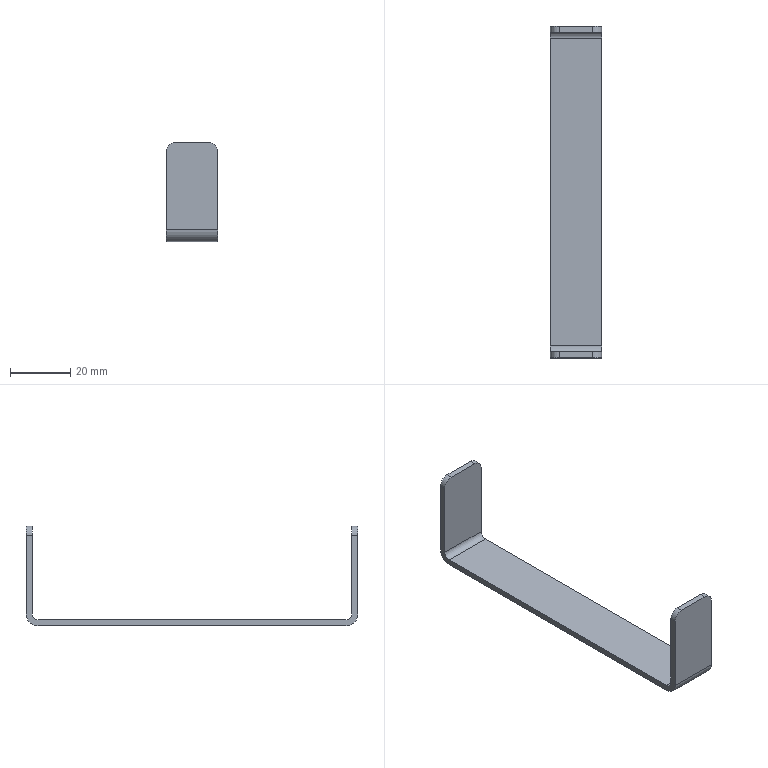Part | NX | features solid 2 | 1 solid | 18 faces | box 17 x 110 x 33 mm | volume 5745 mm3 | plane 10 | cylinder 8 | commonest cylinder face diameters 6 x4 4 x2 8 x2
STEP:
#1=CARTESIAN_POINT('',(1091.5,-530.,943.5));
#2=VERTEX_POINT('',#1);
#3=CARTESIAN_POINT('',(1094.5,-530.,946.5));
#4=VERTEX_POINT('',#3);
#5=CARTESIAN_POINT('',(1094.5,-530.,943.5));
#6=DIRECTION('',(0.,1.,0.));
#7=DIRECTION('',(0.,0.,1.));
#8=AXIS2_PLACEMENT_3D('',#5,#6,#7);
#9=CIRCLE('',#8,3.);
#10=EDGE_CURVE('',#2,#4,#9,.T.);
#11=ORIENTED_EDGE('',*,*,#10,.F.);
#12=CARTESIAN_POINT('',(1091.5,-532.,943.5));
#13=VERTEX_POINT('',#12);
#14=CARTESIAN_POINT('',(1091.5,-422.,943.5));
#15=DIRECTION('',(0.,1.,0.));
#16=VECTOR('',#15,1000.);
#17=LINE('',#14,#16);
#18=EDGE_CURVE('',#13,#2,#17,.T.);
#19=ORIENTED_EDGE('',*,*,#18,.F.);
#20=CARTESIAN_POINT('',(1094.5,-532.,946.5));
#21=VERTEX_POINT('',#20);
#22=CARTESIAN_POINT('',(1094.5,-532.,943.5));
#23=DIRECTION('',(0.,-1.,0.));
#24=DIRECTION('',(0.,0.,1.));
#25=AXIS2_PLACEMENT_3D('',#22,#23,#24);
#26=CIRCLE('',#25,3.);
#27=EDGE_CURVE('',#21,#13,#26,.T.);
#28=ORIENTED_EDGE('',*,*,#27,.F.);
#29=CARTESIAN_POINT('',(1094.5,-532.,946.5));
#30=DIRECTION('',(0.,-1.,0.));
#31=VECTOR('',#30,1000.);
#32=LINE('',#29,#31);
#33=EDGE_CURVE('',#4,#21,#32,.T.);
#34=ORIENTED_EDGE('',*,*,#33,.F.);
#35=EDGE_LOOP('',(#11,#19,#28,#34));
#36=FACE_BOUND('',#35,.T.);
#37=CARTESIAN_POINT('',(1094.5,-532.,943.5));
#38=DIRECTION('',(0.,1.,0.));
#39=DIRECTION('',(0.,0.,-1.));
#40=AXIS2_PLACEMENT_3D('',#37,#38,#39);
#41=CYLINDRICAL_SURFACE('',#40,3.);
#42=ADVANCED_FACE('',(#36),#41,.T.);
#43=CARTESIAN_POINT('',(1105.5,-530.,946.5));
#44=VERTEX_POINT('',#43);
#45=CARTESIAN_POINT('',(1108.5,-530.,943.5));
#46=VERTEX_POINT('',#45);
#47=CARTESIAN_POINT('',(1105.5,-530.,943.5));
#48=DIRECTION('',(0.,1.,0.));
#49=DIRECTION('',(0.,0.,1.));
#50=AXIS2_PLACEMENT_3D('',#47,#48,#49);
#51=CIRCLE('',#50,3.);
#52=EDGE_CURVE('',#44,#46,#51,.T.);
#53=ORIENTED_EDGE('',*,*,#52,.F.);
#54=CARTESIAN_POINT('',(1105.5,-532.,946.5));
#55=VERTEX_POINT('',#54);
#56=CARTESIAN_POINT('',(1105.5,-532.,946.5));
#57=DIRECTION('',(0.,1.,0.));
#58=VECTOR('',#57,1000.);
#59=LINE('',#56,#58);
#60=EDGE_CURVE('',#55,#44,#59,.T.);
#61=ORIENTED_EDGE('',*,*,#60,.F.);
#62=CARTESIAN_POINT('',(1108.5,-532.,943.5));
#63=VERTEX_POINT('',#62);
#64=CARTESIAN_POINT('',(1105.5,-532.,943.5));
#65=DIRECTION('',(0.,-1.,0.));
#66=DIRECTION('',(0.,0.,1.));
#67=AXIS2_PLACEMENT_3D('',#64,#65,#66);
#68=CIRCLE('',#67,3.);
#69=EDGE_CURVE('',#63,#55,#68,.T.);
#70=ORIENTED_EDGE('',*,*,#69,.F.);
#71=CARTESIAN_POINT('',(1108.5,-532.,943.5));
#72=DIRECTION('',(0.,-1.,0.));
#73=VECTOR('',#72,1000.);
#74=LINE('',#71,#73);
#75=EDGE_CURVE('',#46,#63,#74,.T.);
#76=ORIENTED_EDGE('',*,*,#75,.F.);
#77=EDGE_LOOP('',(#53,#61,#70,#76));
#78=FACE_BOUND('',#77,.T.);
#79=CARTESIAN_POINT('',(1105.5,-532.,943.5));
#80=DIRECTION('',(0.,-1.,0.));
#81=DIRECTION('',(0.,0.,1.));
#82=AXIS2_PLACEMENT_3D('',#79,#80,#81);
#83=CYLINDRICAL_SURFACE('',#82,3.);
#84=ADVANCED_FACE('',(#78),#83,.T.);
#85=CARTESIAN_POINT('',(1094.5,-424.,946.5));
#86=VERTEX_POINT('',#85);
#87=CARTESIAN_POINT('',(1091.5,-424.,943.5));
#88=VERTEX_POINT('',#87);
#89=CARTESIAN_POINT('',(1094.5,-424.,943.5));
#90=DIRECTION('',(0.,-1.,0.));
#91=DIRECTION('',(0.,0.,-1.));
#92=AXIS2_PLACEMENT_3D('',#89,#90,#91);
#93=CIRCLE('',#92,3.);
#94=EDGE_CURVE('',#86,#88,#93,.T.);
#95=ORIENTED_EDGE('',*,*,#94,.F.);
#96=CARTESIAN_POINT('',(1094.5,-422.,946.5));
#97=VERTEX_POINT('',#96);
#98=CARTESIAN_POINT('',(1094.5,-422.,946.5));
#99=DIRECTION('',(0.,-1.,0.));
#100=VECTOR('',#99,1000.);
#101=LINE('',#98,#100);
#102=EDGE_CURVE('',#97,#86,#101,.T.);
#103=ORIENTED_EDGE('',*,*,#102,.F.);
#104=CARTESIAN_POINT('',(1091.5,-422.,943.5));
#105=VERTEX_POINT('',#104);
#106=CARTESIAN_POINT('',(1094.5,-422.,943.5));
#107=DIRECTION('',(0.,1.,0.));
#108=DIRECTION('',(0.,0.,-1.));
#109=AXIS2_PLACEMENT_3D('',#106,#107,#108);
#110=CIRCLE('',#109,3.);
#111=EDGE_CURVE('',#105,#97,#110,.T.);
#112=ORIENTED_EDGE('',*,*,#111,.F.);
#113=CARTESIAN_POINT('',(1091.5,-422.,943.5));
#114=DIRECTION('',(0.,1.,0.));
#115=VECTOR('',#114,1000.);
#116=LINE('',#113,#115);
#117=EDGE_CURVE('',#88,#105,#116,.T.);
#118=ORIENTED_EDGE('',*,*,#117,.F.);
#119=EDGE_LOOP('',(#95,#103,#112,#118));
#120=FACE_BOUND('',#119,.T.);
#121=CARTESIAN_POINT('',(1094.5,-422.,943.5));
#122=DIRECTION('',(0.,1.,0.));
#123=DIRECTION('',(0.,0.,-1.));
#124=AXIS2_PLACEMENT_3D('',#121,#122,#123);
#125=CYLINDRICAL_SURFACE('',#124,3.);
#126=ADVANCED_FACE('',(#120),#125,.T.);
#127=CARTESIAN_POINT('',(1108.5,-424.,943.5));
#128=VERTEX_POINT('',#127);
#129=CARTESIAN_POINT('',(1105.5,-424.,946.5));
#130=VERTEX_POINT('',#129);
#131=CARTESIAN_POINT('',(1105.5,-424.,943.5));
#132=DIRECTION('',(0.,-1.,0.));
#133=DIRECTION('',(0.,0.,-1.));
#134=AXIS2_PLACEMENT_3D('',#131,#132,#133);
#135=CIRCLE('',#134,3.);
#136=EDGE_CURVE('',#128,#130,#135,.T.);
#137=ORIENTED_EDGE('',*,*,#136,.F.);
#138=CARTESIAN_POINT('',(1108.5,-422.,943.5));
#139=VERTEX_POINT('',#138);
#140=CARTESIAN_POINT('',(1108.5,-532.,943.5));
#141=DIRECTION('',(0.,-1.,0.));
#142=VECTOR('',#141,1000.);
#143=LINE('',#140,#142);
#144=EDGE_CURVE('',#139,#128,#143,.T.);
#145=ORIENTED_EDGE('',*,*,#144,.F.);
#146=CARTESIAN_POINT('',(1105.5,-422.,946.5));
#147=VERTEX_POINT('',#146);
#148=CARTESIAN_POINT('',(1105.5,-422.,943.5));
#149=DIRECTION('',(0.,1.,0.));
#150=DIRECTION('',(0.,0.,-1.));
#151=AXIS2_PLACEMENT_3D('',#148,#149,#150);
#152=CIRCLE('',#151,3.);
#153=EDGE_CURVE('',#147,#139,#152,.T.);
#154=ORIENTED_EDGE('',*,*,#153,.F.);
#155=CARTESIAN_POINT('',(1105.5,-422.,946.5));
#156=DIRECTION('',(0.,1.,0.));
#157=VECTOR('',#156,1000.);
#158=LINE('',#155,#157);
#159=EDGE_CURVE('',#130,#147,#158,.T.);
#160=ORIENTED_EDGE('',*,*,#159,.F.);
#161=EDGE_LOOP('',(#137,#145,#154,#160));
#162=FACE_BOUND('',#161,.T.);
#163=CARTESIAN_POINT('',(1105.5,-422.,943.5));
#164=DIRECTION('',(0.,-1.,0.));
#165=DIRECTION('',(0.,0.,1.));
#166=AXIS2_PLACEMENT_3D('',#163,#164,#165);
#167=CYLINDRICAL_SURFACE('',#166,3.);
#168=ADVANCED_FACE('',(#162),#167,.T.);
#169=CARTESIAN_POINT('',(1108.5,-424.,917.5));
#170=VERTEX_POINT('',#169);
#171=CARTESIAN_POINT('',(1108.5,-424.,913.5));
#172=DIRECTION('',(0.,0.,1.));
#173=VECTOR('',#172,1000.);
#174=LINE('',#171,#173);
#175=EDGE_CURVE('',#170,#128,#174,.T.);
#176=ORIENTED_EDGE('',*,*,#175,.T.);
#177=ORIENTED_EDGE('',*,*,#136,.T.);
#178=CARTESIAN_POINT('',(1091.5,-424.,946.5));
#179=DIRECTION('',(1.,0.,0.));
#180=VECTOR('',#179,1000.);
#181=LINE('',#178,#180);
#182=EDGE_CURVE('',#86,#130,#181,.T.);
#183=ORIENTED_EDGE('',*,*,#182,.F.);
#184=ORIENTED_EDGE('',*,*,#94,.T.);
#185=CARTESIAN_POINT('',(1091.5,-424.,917.5));
#186=VERTEX_POINT('',#185);
#187=CARTESIAN_POINT('',(1091.5,-424.,913.5));
#188=DIRECTION('',(0.,0.,1.));
#189=VECTOR('',#188,1000.);
#190=LINE('',#187,#189);
#191=EDGE_CURVE('',#186,#88,#190,.T.);
#192=ORIENTED_EDGE('',*,*,#191,.F.);
#193=CARTESIAN_POINT('',(1091.5,-424.,917.5));
#194=DIRECTION('',(1.,0.,0.));
#195=VECTOR('',#194,1000.);
#196=LINE('',#193,#195);
#197=EDGE_CURVE('',#186,#170,#196,.T.);
#198=ORIENTED_EDGE('',*,*,#197,.T.);
#199=EDGE_LOOP('',(#176,#177,#183,#184,#192,#198));
#200=FACE_BOUND('',#199,.T.);
#201=CARTESIAN_POINT('',(1091.5,-424.,913.5));
#202=DIRECTION('',(0.,1.,0.));
#203=DIRECTION('',(0.,0.,-1.));
#204=AXIS2_PLACEMENT_3D('',#201,#202,#203);
#205=PLANE('',#204);
#206=ADVANCED_FACE('',(#200),#205,.F.);
#207=CARTESIAN_POINT('',(1108.5,-426.,915.5));
#208=VERTEX_POINT('',#207);
#209=CARTESIAN_POINT('',(1108.5,-426.,917.5));
#210=DIRECTION('',(1.,0.,0.));
#211=DIRECTION('',(0.,0.,-1.));
#212=AXIS2_PLACEMENT_3D('',#209,#210,#211);
#213=CIRCLE('',#212,2.);
#214=EDGE_CURVE('',#208,#170,#213,.T.);
#215=ORIENTED_EDGE('',*,*,#214,.T.);
#216=ORIENTED_EDGE('',*,*,#197,.F.);
#217=CARTESIAN_POINT('',(1091.5,-426.,915.5));
#218=VERTEX_POINT('',#217);
#219=CARTESIAN_POINT('',(1091.5,-426.,917.5));
#220=DIRECTION('',(1.,0.,0.));
#221=DIRECTION('',(0.,0.,-1.));
#222=AXIS2_PLACEMENT_3D('',#219,#220,#221);
#223=CIRCLE('',#222,2.);
#224=EDGE_CURVE('',#218,#186,#223,.T.);
#225=ORIENTED_EDGE('',*,*,#224,.F.);
#226=CARTESIAN_POINT('',(1091.5,-426.,915.5));
#227=DIRECTION('',(1.,0.,0.));
#228=VECTOR('',#227,1000.);
#229=LINE('',#226,#228);
#230=EDGE_CURVE('',#218,#208,#229,.T.);
#231=ORIENTED_EDGE('',*,*,#230,.T.);
#232=EDGE_LOOP('',(#215,#216,#225,#231));
#233=FACE_BOUND('',#232,.T.);
#234=CARTESIAN_POINT('',(1091.5,-426.,917.5));
#235=DIRECTION('',(1.,0.,0.));
#236=DIRECTION('',(0.,0.,-1.));
#237=AXIS2_PLACEMENT_3D('',#234,#235,#236);
#238=CYLINDRICAL_SURFACE('',#237,2.);
#239=ADVANCED_FACE('',(#233),#238,.F.);
#240=CARTESIAN_POINT('',(1108.5,-528.,915.5));
#241=VERTEX_POINT('',#240);
#242=CARTESIAN_POINT('',(1108.5,-532.,915.5));
#243=DIRECTION('',(0.,1.,0.));
#244=VECTOR('',#243,1000.);
#245=LINE('',#242,#244);
#246=EDGE_CURVE('',#241,#208,#245,.T.);
#247=ORIENTED_EDGE('',*,*,#246,.T.);
#248=ORIENTED_EDGE('',*,*,#230,.F.);
#249=CARTESIAN_POINT('',(1091.5,-528.,915.5));
#250=VERTEX_POINT('',#249);
#251=CARTESIAN_POINT('',(1091.5,-532.,915.5));
#252=DIRECTION('',(0.,1.,0.));
#253=VECTOR('',#252,1000.);
#254=LINE('',#251,#253);
#255=EDGE_CURVE('',#250,#218,#254,.T.);
#256=ORIENTED_EDGE('',*,*,#255,.F.);
#257=CARTESIAN_POINT('',(1091.5,-528.,915.5));
#258=DIRECTION('',(1.,0.,0.));
#259=VECTOR('',#258,1000.);
#260=LINE('',#257,#259);
#261=EDGE_CURVE('',#250,#241,#260,.T.);
#262=ORIENTED_EDGE('',*,*,#261,.T.);
#263=EDGE_LOOP('',(#247,#248,#256,#262));
#264=FACE_BOUND('',#263,.T.);
#265=CARTESIAN_POINT('',(1091.5,-532.,915.5));
#266=DIRECTION('',(0.,0.,-1.));
#267=DIRECTION('',(0.,-1.,0.));
#268=AXIS2_PLACEMENT_3D('',#265,#266,#267);
#269=PLANE('',#268);
#270=ADVANCED_FACE('',(#264),#269,.F.);
#271=CARTESIAN_POINT('',(1108.5,-530.,917.5));
#272=VERTEX_POINT('',#271);
#273=CARTESIAN_POINT('',(1108.5,-528.,917.5));
#274=DIRECTION('',(1.,0.,0.));
#275=DIRECTION('',(0.,0.,-1.));
#276=AXIS2_PLACEMENT_3D('',#273,#274,#275);
#277=CIRCLE('',#276,2.);
#278=EDGE_CURVE('',#272,#241,#277,.T.);
#279=ORIENTED_EDGE('',*,*,#278,.T.);
#280=ORIENTED_EDGE('',*,*,#261,.F.);
#281=CARTESIAN_POINT('',(1091.5,-530.,917.5));
#282=VERTEX_POINT('',#281);
#283=CARTESIAN_POINT('',(1091.5,-528.,917.5));
#284=DIRECTION('',(1.,0.,0.));
#285=DIRECTION('',(0.,0.,-1.));
#286=AXIS2_PLACEMENT_3D('',#283,#284,#285);
#287=CIRCLE('',#286,2.);
#288=EDGE_CURVE('',#282,#250,#287,.T.);
#289=ORIENTED_EDGE('',*,*,#288,.F.);
#290=CARTESIAN_POINT('',(1091.5,-530.,917.5));
#291=DIRECTION('',(1.,0.,0.));
#292=VECTOR('',#291,1000.);
#293=LINE('',#290,#292);
#294=EDGE_CURVE('',#282,#272,#293,.T.);
#295=ORIENTED_EDGE('',*,*,#294,.T.);
#296=EDGE_LOOP('',(#279,#280,#289,#295));
#297=FACE_BOUND('',#296,.T.);
#298=CARTESIAN_POINT('',(1091.5,-528.,917.5));
#299=DIRECTION('',(1.,0.,0.));
#300=DIRECTION('',(0.,0.,-1.));
#301=AXIS2_PLACEMENT_3D('',#298,#299,#300);
#302=CYLINDRICAL_SURFACE('',#301,2.);
#303=ADVANCED_FACE('',(#297),#302,.F.);
#304=CARTESIAN_POINT('',(1091.5,-530.,946.5));
#305=DIRECTION('',(1.,0.,0.));
#306=VECTOR('',#305,1000.);
#307=LINE('',#304,#306);
#308=EDGE_CURVE('',#4,#44,#307,.T.);
#309=ORIENTED_EDGE('',*,*,#308,.T.);
#310=ORIENTED_EDGE('',*,*,#52,.T.);
#311=CARTESIAN_POINT('',(1108.5,-530.,946.5));
#312=DIRECTION('',(0.,0.,-1.));
#313=VECTOR('',#312,1000.);
#314=LINE('',#311,#313);
#315=EDGE_CURVE('',#46,#272,#314,.T.);
#316=ORIENTED_EDGE('',*,*,#315,.T.);
#317=ORIENTED_EDGE('',*,*,#294,.F.);
#318=CARTESIAN_POINT('',(1091.5,-530.,946.5));
#319=DIRECTION('',(0.,0.,-1.));
#320=VECTOR('',#319,1000.);
#321=LINE('',#318,#320);
#322=EDGE_CURVE('',#2,#282,#321,.T.);
#323=ORIENTED_EDGE('',*,*,#322,.F.);
#324=ORIENTED_EDGE('',*,*,#10,.T.);
#325=EDGE_LOOP('',(#309,#310,#316,#317,#323,#324));
#326=FACE_BOUND('',#325,.T.);
#327=CARTESIAN_POINT('',(1091.5,-530.,946.5));
#328=DIRECTION('',(0.,-1.,0.));
#329=DIRECTION('',(0.,0.,-1.));
#330=AXIS2_PLACEMENT_3D('',#327,#328,#329);
#331=PLANE('',#330);
#332=ADVANCED_FACE('',(#326),#331,.F.);
#333=CARTESIAN_POINT('',(1091.5,-422.,946.5));
#334=DIRECTION('',(1.,0.,0.));
#335=VECTOR('',#334,1000.);
#336=LINE('',#333,#335);
#337=EDGE_CURVE('',#97,#147,#336,.T.);
#338=ORIENTED_EDGE('',*,*,#337,.T.);
#339=ORIENTED_EDGE('',*,*,#153,.T.);
#340=CARTESIAN_POINT('',(1108.5,-422.,917.5));
#341=VERTEX_POINT('',#340);
#342=CARTESIAN_POINT('',(1108.5,-422.,913.5));
#343=DIRECTION('',(0.,0.,1.));
#344=VECTOR('',#343,1000.);
#345=LINE('',#342,#344);
#346=EDGE_CURVE('',#341,#139,#345,.T.);
#347=ORIENTED_EDGE('',*,*,#346,.F.);
#348=CARTESIAN_POINT('',(1091.5,-422.,917.5));
#349=VERTEX_POINT('',#348);
#350=CARTESIAN_POINT('',(1091.5,-422.,917.5));
#351=DIRECTION('',(1.,0.,0.));
#352=VECTOR('',#351,1000.);
#353=LINE('',#350,#352);
#354=EDGE_CURVE('',#349,#341,#353,.T.);
#355=ORIENTED_EDGE('',*,*,#354,.F.);
#356=CARTESIAN_POINT('',(1091.5,-422.,913.5));
#357=DIRECTION('',(0.,0.,1.));
#358=VECTOR('',#357,1000.);
#359=LINE('',#356,#358);
#360=EDGE_CURVE('',#349,#105,#359,.T.);
#361=ORIENTED_EDGE('',*,*,#360,.T.);
#362=ORIENTED_EDGE('',*,*,#111,.T.);
#363=EDGE_LOOP('',(#338,#339,#347,#355,#361,#362));
#364=FACE_BOUND('',#363,.T.);
#365=CARTESIAN_POINT('',(1091.5,-422.,913.5));
#366=DIRECTION('',(0.,1.,0.));
#367=DIRECTION('',(0.,0.,-1.));
#368=AXIS2_PLACEMENT_3D('',#365,#366,#367);
#369=PLANE('',#368);
#370=ADVANCED_FACE('',(#364),#369,.T.);
#371=CARTESIAN_POINT('',(1108.5,-426.,913.5));
#372=VERTEX_POINT('',#371);
#373=CARTESIAN_POINT('',(1108.5,-426.,917.5));
#374=DIRECTION('',(1.,0.,0.));
#375=DIRECTION('',(0.,0.,1.));
#376=AXIS2_PLACEMENT_3D('',#373,#374,#375);
#377=CIRCLE('',#376,4.);
#378=EDGE_CURVE('',#372,#341,#377,.T.);
#379=ORIENTED_EDGE('',*,*,#378,.F.);
#380=CARTESIAN_POINT('',(1091.5,-426.,913.5));
#381=VERTEX_POINT('',#380);
#382=CARTESIAN_POINT('',(1091.5,-426.,913.5));
#383=DIRECTION('',(1.,0.,0.));
#384=VECTOR('',#383,1000.);
#385=LINE('',#382,#384);
#386=EDGE_CURVE('',#381,#372,#385,.T.);
#387=ORIENTED_EDGE('',*,*,#386,.F.);
#388=CARTESIAN_POINT('',(1091.5,-426.,917.5));
#389=DIRECTION('',(1.,0.,0.));
#390=DIRECTION('',(0.,0.,1.));
#391=AXIS2_PLACEMENT_3D('',#388,#389,#390);
#392=CIRCLE('',#391,4.);
#393=EDGE_CURVE('',#381,#349,#392,.T.);
#394=ORIENTED_EDGE('',*,*,#393,.T.);
#395=ORIENTED_EDGE('',*,*,#354,.T.);
#396=EDGE_LOOP('',(#379,#387,#394,#395));
#397=FACE_BOUND('',#396,.T.);
#398=CARTESIAN_POINT('',(1091.5,-426.,917.5));
#399=DIRECTION('',(1.,0.,0.));
#400=DIRECTION('',(0.,0.,-1.));
#401=AXIS2_PLACEMENT_3D('',#398,#399,#400);
#402=CYLINDRICAL_SURFACE('',#401,4.);
#403=ADVANCED_FACE('',(#397),#402,.T.);
#404=CARTESIAN_POINT('',(1108.5,-528.,913.5));
#405=VERTEX_POINT('',#404);
#406=CARTESIAN_POINT('',(1108.5,-532.,913.5));
#407=DIRECTION('',(0.,1.,0.));
#408=VECTOR('',#407,1000.);
#409=LINE('',#406,#408);
#410=EDGE_CURVE('',#405,#372,#409,.T.);
#411=ORIENTED_EDGE('',*,*,#410,.F.);
#412=CARTESIAN_POINT('',(1091.5,-528.,913.5));
#413=VERTEX_POINT('',#412);
#414=CARTESIAN_POINT('',(1091.5,-528.,913.5));
#415=DIRECTION('',(1.,0.,0.));
#416=VECTOR('',#415,1000.);
#417=LINE('',#414,#416);
#418=EDGE_CURVE('',#413,#405,#417,.T.);
#419=ORIENTED_EDGE('',*,*,#418,.F.);
#420=CARTESIAN_POINT('',(1091.5,-532.,913.5));
#421=DIRECTION('',(0.,1.,0.));
#422=VECTOR('',#421,1000.);
#423=LINE('',#420,#422);
#424=EDGE_CURVE('',#413,#381,#423,.T.);
#425=ORIENTED_EDGE('',*,*,#424,.T.);
#426=ORIENTED_EDGE('',*,*,#386,.T.);
#427=EDGE_LOOP('',(#411,#419,#425,#426));
#428=FACE_BOUND('',#427,.T.);
#429=CARTESIAN_POINT('',(1091.5,-532.,913.5));
#430=DIRECTION('',(0.,0.,-1.));
#431=DIRECTION('',(0.,-1.,0.));
#432=AXIS2_PLACEMENT_3D('',#429,#430,#431);
#433=PLANE('',#432);
#434=ADVANCED_FACE('',(#428),#433,.T.);
#435=CARTESIAN_POINT('',(1108.5,-532.,917.5));
#436=VERTEX_POINT('',#435);
#437=CARTESIAN_POINT('',(1108.5,-528.,917.5));
#438=DIRECTION('',(1.,0.,0.));
#439=DIRECTION('',(0.,0.,1.));
#440=AXIS2_PLACEMENT_3D('',#437,#438,#439);
#441=CIRCLE('',#440,4.);
#442=EDGE_CURVE('',#436,#405,#441,.T.);
#443=ORIENTED_EDGE('',*,*,#442,.F.);
#444=CARTESIAN_POINT('',(1091.5,-532.,917.5));
#445=VERTEX_POINT('',#444);
#446=CARTESIAN_POINT('',(1091.5,-532.,917.5));
#447=DIRECTION('',(1.,0.,0.));
#448=VECTOR('',#447,1000.);
#449=LINE('',#446,#448);
#450=EDGE_CURVE('',#445,#436,#449,.T.);
#451=ORIENTED_EDGE('',*,*,#450,.F.);
#452=CARTESIAN_POINT('',(1091.5,-528.,917.5));
#453=DIRECTION('',(1.,0.,0.));
#454=DIRECTION('',(0.,0.,1.));
#455=AXIS2_PLACEMENT_3D('',#452,#453,#454);
#456=CIRCLE('',#455,4.);
#457=EDGE_CURVE('',#445,#413,#456,.T.);
#458=ORIENTED_EDGE('',*,*,#457,.T.);
#459=ORIENTED_EDGE('',*,*,#418,.T.);
#460=EDGE_LOOP('',(#443,#451,#458,#459));
#461=FACE_BOUND('',#460,.T.);
#462=CARTESIAN_POINT('',(1091.5,-528.,917.5));
#463=DIRECTION('',(1.,0.,0.));
#464=DIRECTION('',(0.,0.,-1.));
#465=AXIS2_PLACEMENT_3D('',#462,#463,#464);
#466=CYLINDRICAL_SURFACE('',#465,4.);
#467=ADVANCED_FACE('',(#461),#466,.T.);
#468=CARTESIAN_POINT('',(1108.5,-532.,946.5));
#469=DIRECTION('',(0.,0.,-1.));
#470=VECTOR('',#469,1000.);
#471=LINE('',#468,#470);
#472=EDGE_CURVE('',#63,#436,#471,.T.);
#473=ORIENTED_EDGE('',*,*,#472,.F.);
#474=ORIENTED_EDGE('',*,*,#69,.T.);
#475=CARTESIAN_POINT('',(1091.5,-532.,946.5));
#476=DIRECTION('',(1.,0.,0.));
#477=VECTOR('',#476,1000.);
#478=LINE('',#475,#477);
#479=EDGE_CURVE('',#21,#55,#478,.T.);
#480=ORIENTED_EDGE('',*,*,#479,.F.);
#481=ORIENTED_EDGE('',*,*,#27,.T.);
#482=CARTESIAN_POINT('',(1091.5,-532.,946.5));
#483=DIRECTION('',(0.,0.,-1.));
#484=VECTOR('',#483,1000.);
#485=LINE('',#482,#484);
#486=EDGE_CURVE('',#13,#445,#485,.T.);
#487=ORIENTED_EDGE('',*,*,#486,.T.);
#488=ORIENTED_EDGE('',*,*,#450,.T.);
#489=EDGE_LOOP('',(#473,#474,#480,#481,#487,#488));
#490=FACE_BOUND('',#489,.T.);
#491=CARTESIAN_POINT('',(1091.5,-532.,946.5));
#492=DIRECTION('',(0.,-1.,0.));
#493=DIRECTION('',(0.,0.,-1.));
#494=AXIS2_PLACEMENT_3D('',#491,#492,#493);
#495=PLANE('',#494);
#496=ADVANCED_FACE('',(#490),#495,.T.);
#497=ORIENTED_EDGE('',*,*,#479,.T.);
#498=ORIENTED_EDGE('',*,*,#60,.T.);
#499=ORIENTED_EDGE('',*,*,#308,.F.);
#500=ORIENTED_EDGE('',*,*,#33,.T.);
#501=EDGE_LOOP('',(#497,#498,#499,#500));
#502=FACE_BOUND('',#501,.T.);
#503=CARTESIAN_POINT('',(1091.5,-532.,946.5));
#504=DIRECTION('',(0.,0.,-1.));
#505=DIRECTION('',(0.,-1.,0.));
#506=AXIS2_PLACEMENT_3D('',#503,#504,#505);
#507=PLANE('',#506);
#508=ADVANCED_FACE('',(#502),#507,.F.);
#509=ORIENTED_EDGE('',*,*,#346,.T.);
#510=ORIENTED_EDGE('',*,*,#144,.T.);
#511=ORIENTED_EDGE('',*,*,#175,.F.);
#512=ORIENTED_EDGE('',*,*,#214,.F.);
#513=ORIENTED_EDGE('',*,*,#246,.F.);
#514=ORIENTED_EDGE('',*,*,#278,.F.);
#515=ORIENTED_EDGE('',*,*,#315,.F.);
#516=ORIENTED_EDGE('',*,*,#75,.T.);
#517=ORIENTED_EDGE('',*,*,#472,.T.);
#518=ORIENTED_EDGE('',*,*,#442,.T.);
#519=ORIENTED_EDGE('',*,*,#410,.T.);
#520=ORIENTED_EDGE('',*,*,#378,.T.);
#521=EDGE_LOOP('',(#509,#510,#511,#512,#513,#514,#515,#516,#517,#518,#519,#520));
#522=FACE_BOUND('',#521,.T.);
#523=CARTESIAN_POINT('',(1108.5,-532.,946.5));
#524=DIRECTION('',(-1.,0.,0.));
#525=DIRECTION('',(0.,0.,1.));
#526=AXIS2_PLACEMENT_3D('',#523,#524,#525);
#527=PLANE('',#526);
#528=ADVANCED_FACE('',(#522),#527,.F.);
#529=ORIENTED_EDGE('',*,*,#182,.T.);
#530=ORIENTED_EDGE('',*,*,#159,.T.);
#531=ORIENTED_EDGE('',*,*,#337,.F.);
#532=ORIENTED_EDGE('',*,*,#102,.T.);
#533=EDGE_LOOP('',(#529,#530,#531,#532));
#534=FACE_BOUND('',#533,.T.);
#535=CARTESIAN_POINT('',(1091.5,-422.,946.5));
#536=DIRECTION('',(0.,0.,1.));
#537=DIRECTION('',(1.,0.,0.));
#538=AXIS2_PLACEMENT_3D('',#535,#536,#537);
#539=PLANE('',#538);
#540=ADVANCED_FACE('',(#534),#539,.T.);
#541=ORIENTED_EDGE('',*,*,#191,.T.);
#542=ORIENTED_EDGE('',*,*,#117,.T.);
#543=ORIENTED_EDGE('',*,*,#360,.F.);
#544=ORIENTED_EDGE('',*,*,#393,.F.);
#545=ORIENTED_EDGE('',*,*,#424,.F.);
#546=ORIENTED_EDGE('',*,*,#457,.F.);
#547=ORIENTED_EDGE('',*,*,#486,.F.);
#548=ORIENTED_EDGE('',*,*,#18,.T.);
#549=ORIENTED_EDGE('',*,*,#322,.T.);
#550=ORIENTED_EDGE('',*,*,#288,.T.);
#551=ORIENTED_EDGE('',*,*,#255,.T.);
#552=ORIENTED_EDGE('',*,*,#224,.T.);
#553=EDGE_LOOP('',(#541,#542,#543,#544,#545,#546,#547,#548,#549,#550,#551,#552));
#554=FACE_BOUND('',#553,.T.);
#555=CARTESIAN_POINT('',(1091.5,-422.,913.5));
#556=DIRECTION('',(-1.,0.,0.));
#557=DIRECTION('',(0.,0.,1.));
#558=AXIS2_PLACEMENT_3D('',#555,#556,#557);
#559=PLANE('',#558);
#560=ADVANCED_FACE('',(#554),#559,.T.);
#561=CLOSED_SHELL('',(#42,#84,#126,#168,#206,#239,#270,#303,#332,#370,#403,#434,#467,#496,#508,#528,#540,#560));
#562=MANIFOLD_SOLID_BREP('',#561);
#563=(LENGTH_UNIT()NAMED_UNIT(*)SI_UNIT(.MILLI.,.METRE.));
#564=UNCERTAINTY_MEASURE_WITH_UNIT(LENGTH_MEASURE(0.00001),#563,'','');
#565=(NAMED_UNIT(*)PLANE_ANGLE_UNIT()SI_UNIT($,.RADIAN.));
#566=(NAMED_UNIT(*)SI_UNIT($,.STERADIAN.)SOLID_ANGLE_UNIT());
#567=(GEOMETRIC_REPRESENTATION_CONTEXT(3)GLOBAL_UNCERTAINTY_ASSIGNED_CONTEXT((#564))GLOBAL_UNIT_ASSIGNED_CONTEXT((#563,#565,#566))REPRESENTATION_CONTEXT('',''));
#568=ADVANCED_BREP_SHAPE_REPRESENTATION('',(#562),#567);